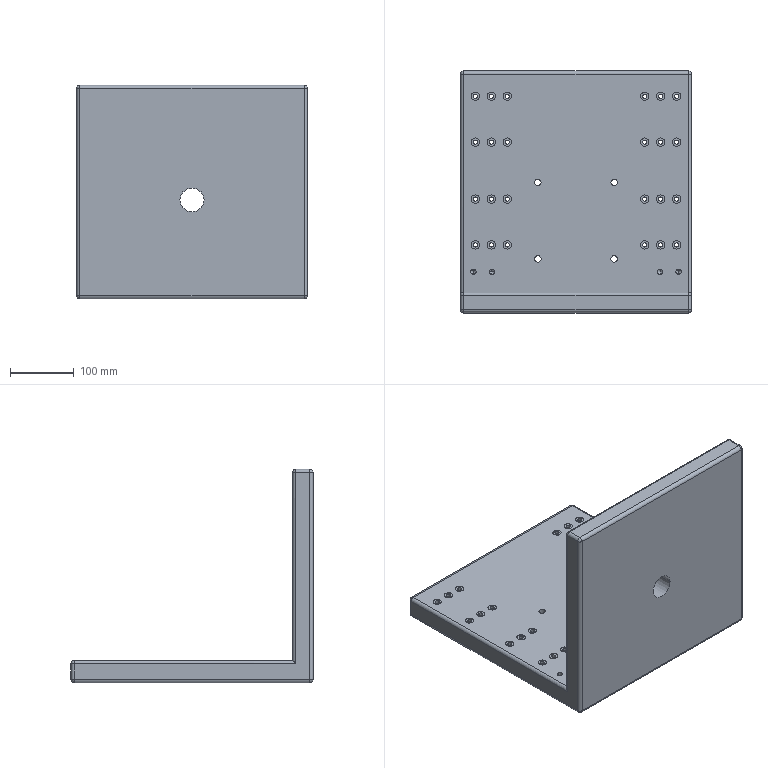Part | STEP file | Fillet 5 | 1 solid | 193 faces | box 363 x 380 x 335 mm | volume 8201164 mm3 | cylinder 137 | plane 32 | cone 14 | sphere 10 | commonest cylinder face diameters 6.6 x48 13 x48 10 x17 8.5 x14 10.2 x8 37.8 x2